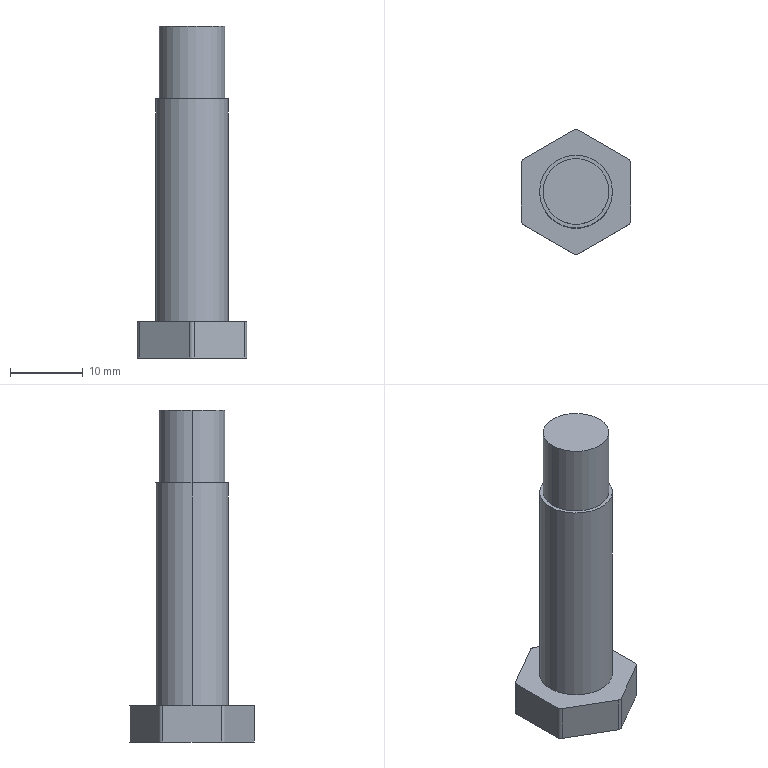Part | STEP file | Screw shaft QY-1-12 | 1 solid | 20 faces | box 15 x 17.135 x 45.5 mm | volume 4005 mm3 | cylinder 10 | plane 10 | commonest cylinder face diameters 1.2 x6 9 x2 10 x2
STEP:
#1=CARTESIAN_POINT('',(0.,0.,0.));
#2=DIRECTION('',(0.,0.,1.));
#3=DIRECTION('',(1.,0.,0.));
#4=AXIS2_PLACEMENT_3D('',#1,#2,#3);
#5=CARTESIAN_POINT('',(4.5,0.,30.5));
#6=VERTEX_POINT('',#5);
#7=CARTESIAN_POINT('',(-4.5,0.,30.5));
#8=VERTEX_POINT('',#7);
#9=CARTESIAN_POINT('',(0.,0.,30.5));
#10=DIRECTION('',(0.,0.,1.));
#11=DIRECTION('',(1.,0.,0.));
#12=AXIS2_PLACEMENT_3D('',#9,#10,#11);
#13=CIRCLE('',#12,4.5);
#14=CARTESIAN_POINT('',(0.,0.,30.5));
#15=DIRECTION('',(0.,0.,1.));
#16=DIRECTION('',(1.,0.,0.));
#17=AXIS2_PLACEMENT_3D('',#14,#15,#16);
#18=CYLINDRICAL_SURFACE('',#17,4.5);
#19=CARTESIAN_POINT('',(0.,0.));
#20=DIRECTION('',(1.,0.));
#21=VECTOR('',#20,1.);
#22=LINE('',#19,#21);
#23=(GEOMETRIC_REPRESENTATION_CONTEXT(2)PARAMETRIC_REPRESENTATION_CONTEXT()REPRESENTATION_CONTEXT('',''));
#24=DEFINITIONAL_REPRESENTATION('',(#22),#23);
#25=PCURVE('',#18,#24);
#26=CARTESIAN_POINT('',(0.,0.,30.5));
#27=DIRECTION('',(0.,0.,1.));
#28=DIRECTION('',(1.,0.,0.));
#29=AXIS2_PLACEMENT_3D('',#26,#27,#28);
#30=PLANE('',#29);
#31=CARTESIAN_POINT('',(0.,0.));
#32=DIRECTION('',(1.,0.));
#33=AXIS2_PLACEMENT_2D('',#31,#32);
#34=CIRCLE('',#33,4.5);
#35=(GEOMETRIC_REPRESENTATION_CONTEXT(2)PARAMETRIC_REPRESENTATION_CONTEXT()REPRESENTATION_CONTEXT('',''));
#36=DEFINITIONAL_REPRESENTATION('',(#34),#35);
#37=PCURVE('',#30,#36);
#38=SURFACE_CURVE('',#13,(#25,#37),.PCURVE_S1.);
#39=EDGE_CURVE('',#6,#8,#38,.T.);
#40=ORIENTED_EDGE('',*,*,#39,.T.);
#41=CARTESIAN_POINT('',(-4.5,0.,40.5));
#42=VERTEX_POINT('',#41);
#43=CARTESIAN_POINT('',(-4.5,0.,30.5));
#44=DIRECTION('',(0.,0.,1.));
#45=VECTOR('',#44,1.);
#46=LINE('',#43,#45);
#47=CARTESIAN_POINT('',(3.142,0.));
#48=DIRECTION('',(0.,1.));
#49=VECTOR('',#48,1.);
#50=LINE('',#47,#49);
#51=(GEOMETRIC_REPRESENTATION_CONTEXT(2)PARAMETRIC_REPRESENTATION_CONTEXT()REPRESENTATION_CONTEXT('',''));
#52=DEFINITIONAL_REPRESENTATION('',(#50),#51);
#53=PCURVE('',#18,#52);
#54=CARTESIAN_POINT('',(0.,0.,30.5));
#55=DIRECTION('',(0.,0.,1.));
#56=DIRECTION('',(1.,0.,0.));
#57=AXIS2_PLACEMENT_3D('',#54,#55,#56);
#58=CYLINDRICAL_SURFACE('',#57,4.5);
#59=CARTESIAN_POINT('',(3.142,0.));
#60=DIRECTION('',(0.,1.));
#61=VECTOR('',#60,1.);
#62=LINE('',#59,#61);
#63=(GEOMETRIC_REPRESENTATION_CONTEXT(2)PARAMETRIC_REPRESENTATION_CONTEXT()REPRESENTATION_CONTEXT('',''));
#64=DEFINITIONAL_REPRESENTATION('',(#62),#63);
#65=PCURVE('',#58,#64);
#66=SURFACE_CURVE('',#46,(#53,#65),.PCURVE_S1.);
#67=EDGE_CURVE('',#8,#42,#66,.T.);
#68=ORIENTED_EDGE('',*,*,#67,.T.);
#69=CARTESIAN_POINT('',(4.5,0.,40.5));
#70=VERTEX_POINT('',#69);
#71=CARTESIAN_POINT('',(0.,0.,40.5));
#72=DIRECTION('',(0.,0.,1.));
#73=DIRECTION('',(1.,0.,0.));
#74=AXIS2_PLACEMENT_3D('',#71,#72,#73);
#75=CIRCLE('',#74,4.5);
#76=CARTESIAN_POINT('',(0.,10.));
#77=DIRECTION('',(1.,0.));
#78=VECTOR('',#77,1.);
#79=LINE('',#76,#78);
#80=(GEOMETRIC_REPRESENTATION_CONTEXT(2)PARAMETRIC_REPRESENTATION_CONTEXT()REPRESENTATION_CONTEXT('',''));
#81=DEFINITIONAL_REPRESENTATION('',(#79),#80);
#82=PCURVE('',#18,#81);
#83=CARTESIAN_POINT('',(0.,0.,40.5));
#84=DIRECTION('',(0.,0.,1.));
#85=DIRECTION('',(1.,0.,0.));
#86=AXIS2_PLACEMENT_3D('',#83,#84,#85);
#87=PLANE('',#86);
#88=CARTESIAN_POINT('',(0.,0.));
#89=DIRECTION('',(1.,0.));
#90=AXIS2_PLACEMENT_2D('',#88,#89);
#91=CIRCLE('',#90,4.5);
#92=(GEOMETRIC_REPRESENTATION_CONTEXT(2)PARAMETRIC_REPRESENTATION_CONTEXT()REPRESENTATION_CONTEXT('',''));
#93=DEFINITIONAL_REPRESENTATION('',(#91),#92);
#94=PCURVE('',#87,#93);
#95=SURFACE_CURVE('',#75,(#82,#94),.PCURVE_S1.);
#96=EDGE_CURVE('',#70,#42,#95,.T.);
#97=ORIENTED_EDGE('',*,*,#96,.F.);
#98=CARTESIAN_POINT('',(4.5,0.,30.5));
#99=DIRECTION('',(0.,0.,1.));
#100=VECTOR('',#99,1.);
#101=LINE('',#98,#100);
#102=CARTESIAN_POINT('',(0.,0.));
#103=DIRECTION('',(0.,1.));
#104=VECTOR('',#103,1.);
#105=LINE('',#102,#104);
#106=(GEOMETRIC_REPRESENTATION_CONTEXT(2)PARAMETRIC_REPRESENTATION_CONTEXT()REPRESENTATION_CONTEXT('',''));
#107=DEFINITIONAL_REPRESENTATION('',(#105),#106);
#108=PCURVE('',#18,#107);
#109=CARTESIAN_POINT('',(6.283,0.));
#110=DIRECTION('',(0.,1.));
#111=VECTOR('',#110,1.);
#112=LINE('',#109,#111);
#113=(GEOMETRIC_REPRESENTATION_CONTEXT(2)PARAMETRIC_REPRESENTATION_CONTEXT()REPRESENTATION_CONTEXT('',''));
#114=DEFINITIONAL_REPRESENTATION('',(#112),#113);
#115=PCURVE('',#58,#114);
#116=SURFACE_CURVE('',#101,(#108,#115),.PCURVE_S1.);
#117=EDGE_CURVE('',#6,#70,#116,.T.);
#118=ORIENTED_EDGE('',*,*,#117,.F.);
#119=EDGE_LOOP('',(#40,#68,#97,#118));
#120=FACE_BOUND('',#119,.T.);
#121=ADVANCED_FACE('',(#120),#18,.T.);
#122=CARTESIAN_POINT('',(5.,0.,30.5));
#123=VERTEX_POINT('',#122);
#124=CARTESIAN_POINT('',(-5.,0.,30.5));
#125=VERTEX_POINT('',#124);
#126=CARTESIAN_POINT('',(0.,0.,30.5));
#127=DIRECTION('',(0.,0.,1.));
#128=DIRECTION('',(1.,0.,0.));
#129=AXIS2_PLACEMENT_3D('',#126,#127,#128);
#130=CIRCLE('',#129,5.);
#131=CARTESIAN_POINT('',(0.,0.,36.5));
#132=DIRECTION('',(0.,0.,-1.));
#133=DIRECTION('',(-1.,0.,0.));
#134=AXIS2_PLACEMENT_3D('',#131,#132,#133);
#135=CYLINDRICAL_SURFACE('',#134,5.);
#136=CARTESIAN_POINT('',(3.142,6.));
#137=DIRECTION('',(-1.,0.));
#138=VECTOR('',#137,1.);
#139=LINE('',#136,#138);
#140=(GEOMETRIC_REPRESENTATION_CONTEXT(2)PARAMETRIC_REPRESENTATION_CONTEXT()REPRESENTATION_CONTEXT('',''));
#141=DEFINITIONAL_REPRESENTATION('',(#139),#140);
#142=PCURVE('',#135,#141);
#143=CARTESIAN_POINT('',(0.,0.));
#144=DIRECTION('',(1.,0.));
#145=AXIS2_PLACEMENT_2D('',#143,#144);
#146=CIRCLE('',#145,5.);
#147=(GEOMETRIC_REPRESENTATION_CONTEXT(2)PARAMETRIC_REPRESENTATION_CONTEXT()REPRESENTATION_CONTEXT('',''));
#148=DEFINITIONAL_REPRESENTATION('',(#146),#147);
#149=PCURVE('',#30,#148);
#150=SURFACE_CURVE('',#130,(#142,#149),.PCURVE_S1.);
#151=EDGE_CURVE('',#123,#125,#150,.T.);
#152=ORIENTED_EDGE('',*,*,#151,.F.);
#153=CARTESIAN_POINT('',(5.,0.,0.));
#154=VERTEX_POINT('',#153);
#155=CARTESIAN_POINT('',(5.,0.,36.5));
#156=DIRECTION('',(0.,0.,-1.));
#157=VECTOR('',#156,1.);
#158=LINE('',#155,#157);
#159=CARTESIAN_POINT('',(3.142,0.));
#160=DIRECTION('',(0.,1.));
#161=VECTOR('',#160,1.);
#162=LINE('',#159,#161);
#163=(GEOMETRIC_REPRESENTATION_CONTEXT(2)PARAMETRIC_REPRESENTATION_CONTEXT()REPRESENTATION_CONTEXT('',''));
#164=DEFINITIONAL_REPRESENTATION('',(#162),#163);
#165=PCURVE('',#135,#164);
#166=CARTESIAN_POINT('',(0.,0.,36.5));
#167=DIRECTION('',(0.,0.,-1.));
#168=DIRECTION('',(-1.,0.,0.));
#169=AXIS2_PLACEMENT_3D('',#166,#167,#168);
#170=CYLINDRICAL_SURFACE('',#169,5.);
#171=CARTESIAN_POINT('',(3.142,0.));
#172=DIRECTION('',(0.,1.));
#173=VECTOR('',#172,1.);
#174=LINE('',#171,#173);
#175=(GEOMETRIC_REPRESENTATION_CONTEXT(2)PARAMETRIC_REPRESENTATION_CONTEXT()REPRESENTATION_CONTEXT('',''));
#176=DEFINITIONAL_REPRESENTATION('',(#174),#175);
#177=PCURVE('',#170,#176);
#178=SURFACE_CURVE('',#158,(#165,#177),.PCURVE_S1.);
#179=EDGE_CURVE('',#123,#154,#178,.T.);
#180=ORIENTED_EDGE('',*,*,#179,.T.);
#181=CARTESIAN_POINT('',(-5.,0.,0.));
#182=VERTEX_POINT('',#181);
#183=CARTESIAN_POINT('',(0.,0.,0.));
#184=DIRECTION('',(0.,0.,1.));
#185=DIRECTION('',(1.,0.,0.));
#186=AXIS2_PLACEMENT_3D('',#183,#184,#185);
#187=CIRCLE('',#186,5.);
#188=CARTESIAN_POINT('',(3.142,36.5));
#189=DIRECTION('',(-1.,0.));
#190=VECTOR('',#189,1.);
#191=LINE('',#188,#190);
#192=(GEOMETRIC_REPRESENTATION_CONTEXT(2)PARAMETRIC_REPRESENTATION_CONTEXT()REPRESENTATION_CONTEXT('',''));
#193=DEFINITIONAL_REPRESENTATION('',(#191),#192);
#194=PCURVE('',#135,#193);
#195=CARTESIAN_POINT('',(-6.9,3.984,0.));
#196=DIRECTION('',(0.,0.,-1.));
#197=DIRECTION('',(-1.,0.,0.));
#198=AXIS2_PLACEMENT_3D('',#195,#196,#197);
#199=PLANE('',#198);
#200=CARTESIAN_POINT('',(-11.9,-3.984));
#201=CARTESIAN_POINT('',(-11.9,4.677));
#202=CARTESIAN_POINT('',(-4.4,0.3464));
#203=CARTESIAN_POINT('',(3.1,-3.984));
#204=CARTESIAN_POINT('',(-4.4,-8.314));
#205=CARTESIAN_POINT('',(-11.9,-12.644));
#206=CARTESIAN_POINT('',(-11.9,-3.984));
#207=(BOUNDED_CURVE()B_SPLINE_CURVE(2,(#200,#201,#202,#203,#204,#205,#206),.UNSPECIFIED.,.T.,.F.)B_SPLINE_CURVE_WITH_KNOTS((1,2,2,2,2,1),(-2.094,0.,2.094,4.189,6.283,8.378),.UNSPECIFIED.)CURVE()GEOMETRIC_REPRESENTATION_ITEM()RATIONAL_B_SPLINE_CURVE((1.,0.5,1.,0.5,1.,0.5,1.))REPRESENTATION_ITEM(''));
#208=(GEOMETRIC_REPRESENTATION_CONTEXT(2)PARAMETRIC_REPRESENTATION_CONTEXT()REPRESENTATION_CONTEXT('',''));
#209=DEFINITIONAL_REPRESENTATION('',(#207),#208);
#210=PCURVE('',#199,#209);
#211=SURFACE_CURVE('',#187,(#194,#210),.PCURVE_S1.);
#212=EDGE_CURVE('',#154,#182,#211,.T.);
#213=ORIENTED_EDGE('',*,*,#212,.T.);
#214=CARTESIAN_POINT('',(-5.,0.,36.5));
#215=DIRECTION('',(0.,0.,-1.));
#216=VECTOR('',#215,1.);
#217=LINE('',#214,#216);
#218=CARTESIAN_POINT('',(0.,0.));
#219=DIRECTION('',(0.,1.));
#220=VECTOR('',#219,1.);
#221=LINE('',#218,#220);
#222=(GEOMETRIC_REPRESENTATION_CONTEXT(2)PARAMETRIC_REPRESENTATION_CONTEXT()REPRESENTATION_CONTEXT('',''));
#223=DEFINITIONAL_REPRESENTATION('',(#221),#222);
#224=PCURVE('',#135,#223);
#225=CARTESIAN_POINT('',(6.283,0.));
#226=DIRECTION('',(0.,1.));
#227=VECTOR('',#226,1.);
#228=LINE('',#225,#227);
#229=(GEOMETRIC_REPRESENTATION_CONTEXT(2)PARAMETRIC_REPRESENTATION_CONTEXT()REPRESENTATION_CONTEXT('',''));
#230=DEFINITIONAL_REPRESENTATION('',(#228),#229);
#231=PCURVE('',#170,#230);
#232=SURFACE_CURVE('',#217,(#224,#231),.PCURVE_S1.);
#233=EDGE_CURVE('',#125,#182,#232,.T.);
#234=ORIENTED_EDGE('',*,*,#233,.F.);
#235=EDGE_LOOP('',(#152,#180,#213,#234));
#236=FACE_BOUND('',#235,.T.);
#237=ADVANCED_FACE('',(#236),#135,.T.);
#238=ORIENTED_EDGE('',*,*,#179,.F.);
#239=CARTESIAN_POINT('',(0.,0.,30.5));
#240=DIRECTION('',(0.,0.,1.));
#241=DIRECTION('',(1.,0.,0.));
#242=AXIS2_PLACEMENT_3D('',#239,#240,#241);
#243=CIRCLE('',#242,5.);
#244=CARTESIAN_POINT('',(9.425,6.));
#245=DIRECTION('',(-1.,0.));
#246=VECTOR('',#245,1.);
#247=LINE('',#244,#246);
#248=(GEOMETRIC_REPRESENTATION_CONTEXT(2)PARAMETRIC_REPRESENTATION_CONTEXT()REPRESENTATION_CONTEXT('',''));
#249=DEFINITIONAL_REPRESENTATION('',(#247),#248);
#250=PCURVE('',#170,#249);
#251=CARTESIAN_POINT('',(0.,0.));
#252=DIRECTION('',(1.,0.));
#253=AXIS2_PLACEMENT_2D('',#251,#252);
#254=CIRCLE('',#253,5.);
#255=(GEOMETRIC_REPRESENTATION_CONTEXT(2)PARAMETRIC_REPRESENTATION_CONTEXT()REPRESENTATION_CONTEXT('',''));
#256=DEFINITIONAL_REPRESENTATION('',(#254),#255);
#257=PCURVE('',#30,#256);
#258=SURFACE_CURVE('',#243,(#250,#257),.PCURVE_S1.);
#259=EDGE_CURVE('',#125,#123,#258,.T.);
#260=ORIENTED_EDGE('',*,*,#259,.F.);
#261=ORIENTED_EDGE('',*,*,#233,.T.);
#262=CARTESIAN_POINT('',(0.,0.,0.));
#263=DIRECTION('',(0.,0.,1.));
#264=DIRECTION('',(1.,0.,0.));
#265=AXIS2_PLACEMENT_3D('',#262,#263,#264);
#266=CIRCLE('',#265,5.);
#267=CARTESIAN_POINT('',(9.425,36.5));
#268=DIRECTION('',(-1.,0.));
#269=VECTOR('',#268,1.);
#270=LINE('',#267,#269);
#271=(GEOMETRIC_REPRESENTATION_CONTEXT(2)PARAMETRIC_REPRESENTATION_CONTEXT()REPRESENTATION_CONTEXT('',''));
#272=DEFINITIONAL_REPRESENTATION('',(#270),#271);
#273=PCURVE('',#170,#272);
#274=CARTESIAN_POINT('',(-11.9,-3.984));
#275=CARTESIAN_POINT('',(-11.9,4.677));
#276=CARTESIAN_POINT('',(-4.4,0.3464));
#277=CARTESIAN_POINT('',(3.1,-3.984));
#278=CARTESIAN_POINT('',(-4.4,-8.314));
#279=CARTESIAN_POINT('',(-11.9,-12.644));
#280=CARTESIAN_POINT('',(-11.9,-3.984));
#281=(BOUNDED_CURVE()B_SPLINE_CURVE(2,(#274,#275,#276,#277,#278,#279,#280),.UNSPECIFIED.,.T.,.F.)B_SPLINE_CURVE_WITH_KNOTS((1,2,2,2,2,1),(-2.094,0.,2.094,4.189,6.283,8.378),.UNSPECIFIED.)CURVE()GEOMETRIC_REPRESENTATION_ITEM()RATIONAL_B_SPLINE_CURVE((1.,0.5,1.,0.5,1.,0.5,1.))REPRESENTATION_ITEM(''));
#282=(GEOMETRIC_REPRESENTATION_CONTEXT(2)PARAMETRIC_REPRESENTATION_CONTEXT()REPRESENTATION_CONTEXT('',''));
#283=DEFINITIONAL_REPRESENTATION('',(#281),#282);
#284=PCURVE('',#199,#283);
#285=SURFACE_CURVE('',#266,(#273,#284),.PCURVE_S1.);
#286=EDGE_CURVE('',#182,#154,#285,.T.);
#287=ORIENTED_EDGE('',*,*,#286,.T.);
#288=EDGE_LOOP('',(#238,#260,#261,#287));
#289=FACE_BOUND('',#288,.T.);
#290=ADVANCED_FACE('',(#289),#170,.T.);
#291=CARTESIAN_POINT('',(-7.5,3.984,0.));
#292=VERTEX_POINT('',#291);
#293=CARTESIAN_POINT('',(-7.2,4.503,0.));
#294=VERTEX_POINT('',#293);
#295=CARTESIAN_POINT('',(-6.9,3.984,0.));
#296=DIRECTION('',(0.,0.,-1.));
#297=DIRECTION('',(-1.,0.,0.));
#298=AXIS2_PLACEMENT_3D('',#295,#296,#297);
#299=CIRCLE('',#298,0.6);
#300=CARTESIAN_POINT('',(-6.9,3.984,-5.));
#301=DIRECTION('',(0.,0.,1.));
#302=DIRECTION('',(1.,0.,0.));
#303=AXIS2_PLACEMENT_3D('',#300,#301,#302);
#304=CYLINDRICAL_SURFACE('',#303,0.6);
#305=CARTESIAN_POINT('',(3.142,5.));
#306=DIRECTION('',(-1.,0.));
#307=VECTOR('',#306,1.);
#308=LINE('',#305,#307);
#309=(GEOMETRIC_REPRESENTATION_CONTEXT(2)PARAMETRIC_REPRESENTATION_CONTEXT()REPRESENTATION_CONTEXT('',''));
#310=DEFINITIONAL_REPRESENTATION('',(#308),#309);
#311=PCURVE('',#304,#310);
#312=CARTESIAN_POINT('',(0.,0.));
#313=DIRECTION('',(1.,0.));
#314=AXIS2_PLACEMENT_2D('',#312,#313);
#315=CIRCLE('',#314,0.6);
#316=(GEOMETRIC_REPRESENTATION_CONTEXT(2)PARAMETRIC_REPRESENTATION_CONTEXT()REPRESENTATION_CONTEXT('',''));
#317=DEFINITIONAL_REPRESENTATION('',(#315),#316);
#318=PCURVE('',#199,#317);
#319=SURFACE_CURVE('',#299,(#311,#318),.PCURVE_S1.);
#320=EDGE_CURVE('',#292,#294,#319,.T.);
#321=ORIENTED_EDGE('',*,*,#320,.T.);
#322=CARTESIAN_POINT('',(-7.2,4.503,-5.));
#323=VERTEX_POINT('',#322);
#324=CARTESIAN_POINT('',(-7.2,4.503,-5.));
#325=DIRECTION('',(0.,0.,1.));
#326=VECTOR('',#325,1.);
#327=LINE('',#324,#326);
#328=CARTESIAN_POINT('',(2.094,0.));
#329=DIRECTION('',(0.,1.));
#330=VECTOR('',#329,1.);
#331=LINE('',#328,#330);
#332=(GEOMETRIC_REPRESENTATION_CONTEXT(2)PARAMETRIC_REPRESENTATION_CONTEXT()REPRESENTATION_CONTEXT('',''));
#333=DEFINITIONAL_REPRESENTATION('',(#331),#332);
#334=PCURVE('',#304,#333);
#335=CARTESIAN_POINT('',(-7.2,4.503,-5.));
#336=DIRECTION('',(0.5,-0.866,0.));
#337=DIRECTION('',(0.866,0.5,0.));
#338=AXIS2_PLACEMENT_3D('',#335,#336,#337);
#339=PLANE('',#338);
#340=CARTESIAN_POINT('',(0.,0.));
#341=DIRECTION('',(0.,1.));
#342=VECTOR('',#341,1.);
#343=LINE('',#340,#342);
#344=(GEOMETRIC_REPRESENTATION_CONTEXT(2)PARAMETRIC_REPRESENTATION_CONTEXT()REPRESENTATION_CONTEXT('',''));
#345=DEFINITIONAL_REPRESENTATION('',(#343),#344);
#346=PCURVE('',#339,#345);
#347=SURFACE_CURVE('',#327,(#334,#346),.PCURVE_S1.);
#348=EDGE_CURVE('',#323,#294,#347,.T.);
#349=ORIENTED_EDGE('',*,*,#348,.F.);
#350=CARTESIAN_POINT('',(-7.5,3.984,-5.));
#351=VERTEX_POINT('',#350);
#352=CARTESIAN_POINT('',(-6.9,3.984,-5.));
#353=DIRECTION('',(0.,0.,-1.));
#354=DIRECTION('',(-1.,0.,0.));
#355=AXIS2_PLACEMENT_3D('',#352,#353,#354);
#356=CIRCLE('',#355,0.6);
#357=CARTESIAN_POINT('',(3.142,0.));
#358=DIRECTION('',(-1.,0.));
#359=VECTOR('',#358,1.);
#360=LINE('',#357,#359);
#361=(GEOMETRIC_REPRESENTATION_CONTEXT(2)PARAMETRIC_REPRESENTATION_CONTEXT()REPRESENTATION_CONTEXT('',''));
#362=DEFINITIONAL_REPRESENTATION('',(#360),#361);
#363=PCURVE('',#304,#362);
#364=CARTESIAN_POINT('',(-6.9,3.984,-5.));
#365=DIRECTION('',(0.,0.,-1.));
#366=DIRECTION('',(-1.,0.,0.));
#367=AXIS2_PLACEMENT_3D('',#364,#365,#366);
#368=PLANE('',#367);
#369=CARTESIAN_POINT('',(0.,0.));
#370=DIRECTION('',(1.,0.));
#371=AXIS2_PLACEMENT_2D('',#369,#370);
#372=CIRCLE('',#371,0.6);
#373=(GEOMETRIC_REPRESENTATION_CONTEXT(2)PARAMETRIC_REPRESENTATION_CONTEXT()REPRESENTATION_CONTEXT('',''));
#374=DEFINITIONAL_REPRESENTATION('',(#372),#373);
#375=PCURVE('',#368,#374);
#376=SURFACE_CURVE('',#356,(#363,#375),.PCURVE_S1.);
#377=EDGE_CURVE('',#351,#323,#376,.T.);
#378=ORIENTED_EDGE('',*,*,#377,.F.);
#379=CARTESIAN_POINT('',(-7.5,3.984,-5.));
#380=DIRECTION('',(0.,0.,1.));
#381=VECTOR('',#380,1.);
#382=LINE('',#379,#381);
#383=CARTESIAN_POINT('',(3.142,0.));
#384=DIRECTION('',(0.,1.));
#385=VECTOR('',#384,1.);
#386=LINE('',#383,#385);
#387=(GEOMETRIC_REPRESENTATION_CONTEXT(2)PARAMETRIC_REPRESENTATION_CONTEXT()REPRESENTATION_CONTEXT('',''));
#388=DEFINITIONAL_REPRESENTATION('',(#386),#387);
#389=PCURVE('',#304,#388);
#390=CARTESIAN_POINT('',(-7.5,-3.984,-5.));
#391=DIRECTION('',(1.,0.,0.));
#392=DIRECTION('',(0.,1.,0.));
#393=AXIS2_PLACEMENT_3D('',#390,#391,#392);
#394=PLANE('',#393);
#395=CARTESIAN_POINT('',(7.967,0.));
#396=DIRECTION('',(0.,1.));
#397=VECTOR('',#396,1.);
#398=LINE('',#395,#397);
#399=(GEOMETRIC_REPRESENTATION_CONTEXT(2)PARAMETRIC_REPRESENTATION_CONTEXT()REPRESENTATION_CONTEXT('',''));
#400=DEFINITIONAL_REPRESENTATION('',(#398),#399);
#401=PCURVE('',#394,#400);
#402=SURFACE_CURVE('',#382,(#389,#401),.PCURVE_S1.);
#403=EDGE_CURVE('',#351,#292,#402,.T.);
#404=ORIENTED_EDGE('',*,*,#403,.T.);
#405=EDGE_LOOP('',(#321,#349,#378,#404));
#406=FACE_BOUND('',#405,.T.);
#407=ADVANCED_FACE('',(#406),#304,.T.);
#408=CARTESIAN_POINT('',(-0.3,8.487,0.));
#409=VERTEX_POINT('',#408);
#410=CARTESIAN_POINT('',(-7.2,4.503,0.));
#411=DIRECTION('',(0.866,0.5,0.));
#412=VECTOR('',#411,1.);
#413=LINE('',#410,#412);
#414=CARTESIAN_POINT('',(0.,5.));
#415=DIRECTION('',(1.,0.));
#416=VECTOR('',#415,1.);
#417=LINE('',#414,#416);
#418=(GEOMETRIC_REPRESENTATION_CONTEXT(2)PARAMETRIC_REPRESENTATION_CONTEXT()REPRESENTATION_CONTEXT('',''));
#419=DEFINITIONAL_REPRESENTATION('',(#417),#418);
#420=PCURVE('',#339,#419);
#421=CARTESIAN_POINT('',(0.3,0.5196));
#422=DIRECTION('',(-0.866,0.5));
#423=VECTOR('',#422,1.);
#424=LINE('',#421,#423);
#425=(GEOMETRIC_REPRESENTATION_CONTEXT(2)PARAMETRIC_REPRESENTATION_CONTEXT()REPRESENTATION_CONTEXT('',''));
#426=DEFINITIONAL_REPRESENTATION('',(#424),#425);
#427=PCURVE('',#199,#426);
#428=SURFACE_CURVE('',#413,(#420,#427),.PCURVE_S1.);
#429=EDGE_CURVE('',#294,#409,#428,.T.);
#430=ORIENTED_EDGE('',*,*,#429,.T.);
#431=CARTESIAN_POINT('',(-0.3,8.487,-5.));
#432=VERTEX_POINT('',#431);
#433=CARTESIAN_POINT('',(-0.3,8.487,-5.));
#434=DIRECTION('',(0.,0.,1.));
#435=VECTOR('',#434,1.);
#436=LINE('',#433,#435);
#437=CARTESIAN_POINT('',(7.967,0.));
#438=DIRECTION('',(0.,1.));
#439=VECTOR('',#438,1.);
#440=LINE('',#437,#439);
#441=(GEOMETRIC_REPRESENTATION_CONTEXT(2)PARAMETRIC_REPRESENTATION_CONTEXT()REPRESENTATION_CONTEXT('',''));
#442=DEFINITIONAL_REPRESENTATION('',(#440),#441);
#443=PCURVE('',#339,#442);
#444=CARTESIAN_POINT('',(0.,7.967,-5.));
#445=DIRECTION('',(0.,0.,1.));
#446=DIRECTION('',(1.,0.,0.));
#447=AXIS2_PLACEMENT_3D('',#444,#445,#446);
#448=CYLINDRICAL_SURFACE('',#447,0.6);
#449=CARTESIAN_POINT('',(2.094,0.));
#450=DIRECTION('',(0.,1.));
#451=VECTOR('',#450,1.);
#452=LINE('',#449,#451);
#453=(GEOMETRIC_REPRESENTATION_CONTEXT(2)PARAMETRIC_REPRESENTATION_CONTEXT()REPRESENTATION_CONTEXT('',''));
#454=DEFINITIONAL_REPRESENTATION('',(#452),#453);
#455=PCURVE('',#448,#454);
#456=SURFACE_CURVE('',#436,(#443,#455),.PCURVE_S1.);
#457=EDGE_CURVE('',#432,#409,#456,.T.);
#458=ORIENTED_EDGE('',*,*,#457,.F.);
#459=CARTESIAN_POINT('',(-7.2,4.503,-5.));
#460=DIRECTION('',(0.866,0.5,0.));
#461=VECTOR('',#460,1.);
#462=LINE('',#459,#461);
#463=CARTESIAN_POINT('',(0.,0.));
#464=DIRECTION('',(1.,0.));
#465=VECTOR('',#464,1.);
#466=LINE('',#463,#465);
#467=(GEOMETRIC_REPRESENTATION_CONTEXT(2)PARAMETRIC_REPRESENTATION_CONTEXT()REPRESENTATION_CONTEXT('',''));
#468=DEFINITIONAL_REPRESENTATION('',(#466),#467);
#469=PCURVE('',#339,#468);
#470=CARTESIAN_POINT('',(0.3,0.5196));
#471=DIRECTION('',(-0.866,0.5));
#472=VECTOR('',#471,1.);
#473=LINE('',#470,#472);
#474=(GEOMETRIC_REPRESENTATION_CONTEXT(2)PARAMETRIC_REPRESENTATION_CONTEXT()REPRESENTATION_CONTEXT('',''));
#475=DEFINITIONAL_REPRESENTATION('',(#473),#474);
#476=PCURVE('',#368,#475);
#477=SURFACE_CURVE('',#462,(#469,#476),.PCURVE_S1.);
#478=EDGE_CURVE('',#323,#432,#477,.T.);
#479=ORIENTED_EDGE('',*,*,#478,.F.);
#480=ORIENTED_EDGE('',*,*,#348,.T.);
#481=EDGE_LOOP('',(#430,#458,#479,#480));
#482=FACE_BOUND('',#481,.T.);
#483=ADVANCED_FACE('',(#482),#339,.F.);
#484=CARTESIAN_POINT('',(0.3,8.487,0.));
#485=VERTEX_POINT('',#484);
#486=CARTESIAN_POINT('',(0.,7.967,0.));
#487=DIRECTION('',(0.,0.,-1.));
#488=DIRECTION('',(1.,0.,0.));
#489=AXIS2_PLACEMENT_3D('',#486,#487,#488);
#490=CIRCLE('',#489,0.6);
#491=CARTESIAN_POINT('',(6.283,5.));
#492=DIRECTION('',(-1.,0.));
#493=VECTOR('',#492,1.);
#494=LINE('',#491,#493);
#495=(GEOMETRIC_REPRESENTATION_CONTEXT(2)PARAMETRIC_REPRESENTATION_CONTEXT()REPRESENTATION_CONTEXT('',''));
#496=DEFINITIONAL_REPRESENTATION('',(#494),#495);
#497=PCURVE('',#448,#496);
#498=CARTESIAN_POINT('',(-6.9,3.984));
#499=DIRECTION('',(-1.,0.));
#500=AXIS2_PLACEMENT_2D('',#498,#499);
#501=CIRCLE('',#500,0.6);
#502=(GEOMETRIC_REPRESENTATION_CONTEXT(2)PARAMETRIC_REPRESENTATION_CONTEXT()REPRESENTATION_CONTEXT('',''));
#503=DEFINITIONAL_REPRESENTATION('',(#501),#502);
#504=PCURVE('',#199,#503);
#505=SURFACE_CURVE('',#490,(#497,#504),.PCURVE_S1.);
#506=EDGE_CURVE('',#409,#485,#505,.T.);
#507=ORIENTED_EDGE('',*,*,#506,.T.);
#508=CARTESIAN_POINT('',(0.3,8.487,-5.));
#509=VERTEX_POINT('',#508);
#510=CARTESIAN_POINT('',(0.3,8.487,-5.));
#511=DIRECTION('',(0.,0.,1.));
#512=VECTOR('',#511,1.);
#513=LINE('',#510,#512);
#514=CARTESIAN_POINT('',(1.047,0.));
#515=DIRECTION('',(0.,1.));
#516=VECTOR('',#515,1.);
#517=LINE('',#514,#516);
#518=(GEOMETRIC_REPRESENTATION_CONTEXT(2)PARAMETRIC_REPRESENTATION_CONTEXT()REPRESENTATION_CONTEXT('',''));
#519=DEFINITIONAL_REPRESENTATION('',(#517),#518);
#520=PCURVE('',#448,#519);
#521=CARTESIAN_POINT('',(0.3,8.487,-5.));
#522=DIRECTION('',(-0.5,-0.866,0.));
#523=DIRECTION('',(0.866,-0.5,0.));
#524=AXIS2_PLACEMENT_3D('',#521,#522,#523);
#525=PLANE('',#524);
#526=CARTESIAN_POINT('',(0.,0.));
#527=DIRECTION('',(0.,1.));
#528=VECTOR('',#527,1.);
#529=LINE('',#526,#528);
#530=(GEOMETRIC_REPRESENTATION_CONTEXT(2)PARAMETRIC_REPRESENTATION_CONTEXT()REPRESENTATION_CONTEXT('',''));
#531=DEFINITIONAL_REPRESENTATION('',(#529),#530);
#532=PCURVE('',#525,#531);
#533=SURFACE_CURVE('',#513,(#520,#532),.PCURVE_S1.);
#534=EDGE_CURVE('',#509,#485,#533,.T.);
#535=ORIENTED_EDGE('',*,*,#534,.F.);
#536=CARTESIAN_POINT('',(0.,7.967,-5.));
#537=DIRECTION('',(0.,0.,-1.));
#538=DIRECTION('',(1.,0.,0.));
#539=AXIS2_PLACEMENT_3D('',#536,#537,#538);
#540=CIRCLE('',#539,0.6);
#541=CARTESIAN_POINT('',(6.283,0.));
#542=DIRECTION('',(-1.,0.));
#543=VECTOR('',#542,1.);
#544=LINE('',#541,#543);
#545=(GEOMETRIC_REPRESENTATION_CONTEXT(2)PARAMETRIC_REPRESENTATION_CONTEXT()REPRESENTATION_CONTEXT('',''));
#546=DEFINITIONAL_REPRESENTATION('',(#544),#545);
#547=PCURVE('',#448,#546);
#548=CARTESIAN_POINT('',(-6.9,3.984));
#549=DIRECTION('',(-1.,0.));
#550=AXIS2_PLACEMENT_2D('',#548,#549);
#551=CIRCLE('',#550,0.6);
#552=(GEOMETRIC_REPRESENTATION_CONTEXT(2)PARAMETRIC_REPRESENTATION_CONTEXT()REPRESENTATION_CONTEXT('',''));
#553=DEFINITIONAL_REPRESENTATION('',(#551),#552);
#554=PCURVE('',#368,#553);
#555=SURFACE_CURVE('',#540,(#547,#554),.PCURVE_S1.);
#556=EDGE_CURVE('',#432,#509,#555,.T.);
#557=ORIENTED_EDGE('',*,*,#556,.F.);
#558=ORIENTED_EDGE('',*,*,#457,.T.);
#559=EDGE_LOOP('',(#507,#535,#557,#558));
#560=FACE_BOUND('',#559,.T.);
#561=ADVANCED_FACE('',(#560),#448,.T.);
#562=CARTESIAN_POINT('',(7.2,4.503,0.));
#563=VERTEX_POINT('',#562);
#564=CARTESIAN_POINT('',(0.3,8.487,0.));
#565=DIRECTION('',(0.866,-0.5,0.));
#566=VECTOR('',#565,1.);
#567=LINE('',#564,#566);
#568=CARTESIAN_POINT('',(0.,5.));
#569=DIRECTION('',(1.,0.));
#570=VECTOR('',#569,1.);
#571=LINE('',#568,#570);
#572=(GEOMETRIC_REPRESENTATION_CONTEXT(2)PARAMETRIC_REPRESENTATION_CONTEXT()REPRESENTATION_CONTEXT('',''));
#573=DEFINITIONAL_REPRESENTATION('',(#571),#572);
#574=PCURVE('',#525,#573);
#575=CARTESIAN_POINT('',(-7.2,4.503));
#576=DIRECTION('',(-0.866,-0.5));
#577=VECTOR('',#576,1.);
#578=LINE('',#575,#577);
#579=(GEOMETRIC_REPRESENTATION_CONTEXT(2)PARAMETRIC_REPRESENTATION_CONTEXT()REPRESENTATION_CONTEXT('',''));
#580=DEFINITIONAL_REPRESENTATION('',(#578),#579);
#581=PCURVE('',#199,#580);
#582=SURFACE_CURVE('',#567,(#574,#581),.PCURVE_S1.);
#583=EDGE_CURVE('',#485,#563,#582,.T.);
#584=ORIENTED_EDGE('',*,*,#583,.T.);
#585=CARTESIAN_POINT('',(7.2,4.503,-5.));
#586=VERTEX_POINT('',#585);
#587=CARTESIAN_POINT('',(7.2,4.503,-5.));
#588=DIRECTION('',(0.,0.,1.));
#589=VECTOR('',#588,1.);
#590=LINE('',#587,#589);
#591=CARTESIAN_POINT('',(7.967,0.));
#592=DIRECTION('',(0.,1.));
#593=VECTOR('',#592,1.);
#594=LINE('',#591,#593);
#595=(GEOMETRIC_REPRESENTATION_CONTEXT(2)PARAMETRIC_REPRESENTATION_CONTEXT()REPRESENTATION_CONTEXT('',''));
#596=DEFINITIONAL_REPRESENTATION('',(#594),#595);
#597=PCURVE('',#525,#596);
#598=CARTESIAN_POINT('',(6.9,3.984,-5.));
#599=DIRECTION('',(0.,0.,1.));
#600=DIRECTION('',(1.,0.,0.));
#601=AXIS2_PLACEMENT_3D('',#598,#599,#600);
#602=CYLINDRICAL_SURFACE('',#601,0.6);
#603=CARTESIAN_POINT('',(1.047,0.));
#604=DIRECTION('',(0.,1.));
#605=VECTOR('',#604,1.);
#606=LINE('',#603,#605);
#607=(GEOMETRIC_REPRESENTATION_CONTEXT(2)PARAMETRIC_REPRESENTATION_CONTEXT()REPRESENTATION_CONTEXT('',''));
#608=DEFINITIONAL_REPRESENTATION('',(#606),#607);
#609=PCURVE('',#602,#608);
#610=SURFACE_CURVE('',#590,(#597,#609),.PCURVE_S1.);
#611=EDGE_CURVE('',#586,#563,#610,.T.);
#612=ORIENTED_EDGE('',*,*,#611,.F.);
#613=CARTESIAN_POINT('',(0.3,8.487,-5.));
#614=DIRECTION('',(0.866,-0.5,0.));
#615=VECTOR('',#614,1.);
#616=LINE('',#613,#615);
#617=CARTESIAN_POINT('',(0.,0.));
#618=DIRECTION('',(1.,0.));
#619=VECTOR('',#618,1.);
#620=LINE('',#617,#619);
#621=(GEOMETRIC_REPRESENTATION_CONTEXT(2)PARAMETRIC_REPRESENTATION_CONTEXT()REPRESENTATION_CONTEXT('',''));
#622=DEFINITIONAL_REPRESENTATION('',(#620),#621);
#623=PCURVE('',#525,#622);
#624=CARTESIAN_POINT('',(-7.2,4.503));
#625=DIRECTION('',(-0.866,-0.5));
#626=VECTOR('',#625,1.);
#627=LINE('',#624,#626);
#628=(GEOMETRIC_REPRESENTATION_CONTEXT(2)PARAMETRIC_REPRESENTATION_CONTEXT()REPRESENTATION_CONTEXT('',''));
#629=DEFINITIONAL_REPRESENTATION('',(#627),#628);
#630=PCURVE('',#368,#629);
#631=SURFACE_CURVE('',#616,(#623,#630),.PCURVE_S1.);
#632=EDGE_CURVE('',#509,#586,#631,.T.);
#633=ORIENTED_EDGE('',*,*,#632,.F.);
#634=ORIENTED_EDGE('',*,*,#534,.T.);
#635=EDGE_LOOP('',(#584,#612,#633,#634));
#636=FACE_BOUND('',#635,.T.);
#637=ADVANCED_FACE('',(#636),#525,.F.);
#638=CARTESIAN_POINT('',(7.5,3.984,0.));
#639=VERTEX_POINT('',#638);
#640=CARTESIAN_POINT('',(6.9,3.984,0.));
#641=DIRECTION('',(0.,0.,-1.));
#642=DIRECTION('',(-1.,0.,0.));
#643=AXIS2_PLACEMENT_3D('',#640,#641,#642);
#644=CIRCLE('',#643,0.6);
#645=CARTESIAN_POINT('',(3.142,5.));
#646=DIRECTION('',(-1.,0.));
#647=VECTOR('',#646,1.);
#648=LINE('',#645,#647);
#649=(GEOMETRIC_REPRESENTATION_CONTEXT(2)PARAMETRIC_REPRESENTATION_CONTEXT()REPRESENTATION_CONTEXT('',''));
#650=DEFINITIONAL_REPRESENTATION('',(#648),#649);
#651=PCURVE('',#602,#650);
#652=CARTESIAN_POINT('',(-13.8,0.));
#653=DIRECTION('',(1.,0.));
#654=AXIS2_PLACEMENT_2D('',#652,#653);
#655=CIRCLE('',#654,0.6);
#656=(GEOMETRIC_REPRESENTATION_CONTEXT(2)PARAMETRIC_REPRESENTATION_CONTEXT()REPRESENTATION_CONTEXT('',''));
#657=DEFINITIONAL_REPRESENTATION('',(#655),#656);
#658=PCURVE('',#199,#657);
#659=SURFACE_CURVE('',#644,(#651,#658),.PCURVE_S1.);
#660=EDGE_CURVE('',#563,#639,#659,.T.);
#661=ORIENTED_EDGE('',*,*,#660,.T.);
#662=CARTESIAN_POINT('',(7.5,3.984,-5.));
#663=VERTEX_POINT('',#662);
#664=CARTESIAN_POINT('',(7.5,3.984,-5.));
#665=DIRECTION('',(0.,0.,1.));
#666=VECTOR('',#665,1.);
#667=LINE('',#664,#666);
#668=CARTESIAN_POINT('',(0.,0.));
#669=DIRECTION('',(0.,1.));
#670=VECTOR('',#669,1.);
#671=LINE('',#668,#670);
#672=(GEOMETRIC_REPRESENTATION_CONTEXT(2)PARAMETRIC_REPRESENTATION_CONTEXT()REPRESENTATION_CONTEXT('',''));
#673=DEFINITIONAL_REPRESENTATION('',(#671),#672);
#674=PCURVE('',#602,#673);
#675=CARTESIAN_POINT('',(7.5,3.984,-5.));
#676=DIRECTION('',(-1.,0.,0.));
#677=DIRECTION('',(0.,-1.,0.));
#678=AXIS2_PLACEMENT_3D('',#675,#676,#677);
#679=PLANE('',#678);
#680=CARTESIAN_POINT('',(0.,0.));
#681=DIRECTION('',(0.,1.));
#682=VECTOR('',#681,1.);
#683=LINE('',#680,#682);
#684=(GEOMETRIC_REPRESENTATION_CONTEXT(2)PARAMETRIC_REPRESENTATION_CONTEXT()REPRESENTATION_CONTEXT('',''));
#685=DEFINITIONAL_REPRESENTATION('',(#683),#684);
#686=PCURVE('',#679,#685);
#687=SURFACE_CURVE('',#667,(#674,#686),.PCURVE_S1.);
#688=EDGE_CURVE('',#663,#639,#687,.T.);
#689=ORIENTED_EDGE('',*,*,#688,.F.);
#690=CARTESIAN_POINT('',(6.9,3.984,-5.));
#691=DIRECTION('',(0.,0.,-1.));
#692=DIRECTION('',(-1.,0.,0.));
#693=AXIS2_PLACEMENT_3D('',#690,#691,#692);
#694=CIRCLE('',#693,0.6);
#695=CARTESIAN_POINT('',(3.142,0.));
#696=DIRECTION('',(-1.,0.));
#697=VECTOR('',#696,1.);
#698=LINE('',#695,#697);
#699=(GEOMETRIC_REPRESENTATION_CONTEXT(2)PARAMETRIC_REPRESENTATION_CONTEXT()REPRESENTATION_CONTEXT('',''));
#700=DEFINITIONAL_REPRESENTATION('',(#698),#699);
#701=PCURVE('',#602,#700);
#702=CARTESIAN_POINT('',(-13.8,0.));
#703=DIRECTION('',(1.,0.));
#704=AXIS2_PLACEMENT_2D('',#702,#703);
#705=CIRCLE('',#704,0.6);
#706=(GEOMETRIC_REPRESENTATION_CONTEXT(2)PARAMETRIC_REPRESENTATION_CONTEXT()REPRESENTATION_CONTEXT('',''));
#707=DEFINITIONAL_REPRESENTATION('',(#705),#706);
#708=PCURVE('',#368,#707);
#709=SURFACE_CURVE('',#694,(#701,#708),.PCURVE_S1.);
#710=EDGE_CURVE('',#586,#663,#709,.T.);
#711=ORIENTED_EDGE('',*,*,#710,.F.);
#712=ORIENTED_EDGE('',*,*,#611,.T.);
#713=EDGE_LOOP('',(#661,#689,#711,#712));
#714=FACE_BOUND('',#713,.T.);
#715=ADVANCED_FACE('',(#714),#602,.T.);
#716=CARTESIAN_POINT('',(7.5,-3.984,0.));
#717=VERTEX_POINT('',#716);
#718=CARTESIAN_POINT('',(7.5,3.984,0.));
#719=DIRECTION('',(0.,-1.,0.));
#720=VECTOR('',#719,1.);
#721=LINE('',#718,#720);
#722=CARTESIAN_POINT('',(0.,5.));
#723=DIRECTION('',(1.,0.));
#724=VECTOR('',#723,1.);
#725=LINE('',#722,#724);
#726=(GEOMETRIC_REPRESENTATION_CONTEXT(2)PARAMETRIC_REPRESENTATION_CONTEXT()REPRESENTATION_CONTEXT('',''));
#727=DEFINITIONAL_REPRESENTATION('',(#725),#726);
#728=PCURVE('',#679,#727);
#729=CARTESIAN_POINT('',(-14.4,0.));
#730=DIRECTION('',(0.,-1.));
#731=VECTOR('',#730,1.);
#732=LINE('',#729,#731);
#733=(GEOMETRIC_REPRESENTATION_CONTEXT(2)PARAMETRIC_REPRESENTATION_CONTEXT()REPRESENTATION_CONTEXT('',''));
#734=DEFINITIONAL_REPRESENTATION('',(#732),#733);
#735=PCURVE('',#199,#734);
#736=SURFACE_CURVE('',#721,(#728,#735),.PCURVE_S1.);
#737=EDGE_CURVE('',#639,#717,#736,.T.);
#738=ORIENTED_EDGE('',*,*,#737,.T.);
#739=CARTESIAN_POINT('',(7.5,-3.984,-5.));
#740=VERTEX_POINT('',#739);
#741=CARTESIAN_POINT('',(7.5,-3.984,-5.));
#742=DIRECTION('',(0.,0.,1.));
#743=VECTOR('',#742,1.);
#744=LINE('',#741,#743);
#745=CARTESIAN_POINT('',(7.967,0.));
#746=DIRECTION('',(0.,1.));
#747=VECTOR('',#746,1.);
#748=LINE('',#745,#747);
#749=(GEOMETRIC_REPRESENTATION_CONTEXT(2)PARAMETRIC_REPRESENTATION_CONTEXT()REPRESENTATION_CONTEXT('',''));
#750=DEFINITIONAL_REPRESENTATION('',(#748),#749);
#751=PCURVE('',#679,#750);
#752=CARTESIAN_POINT('',(6.9,-3.984,-5.));
#753=DIRECTION('',(0.,0.,1.));
#754=DIRECTION('',(1.,0.,0.));
#755=AXIS2_PLACEMENT_3D('',#752,#753,#754);
#756=CYLINDRICAL_SURFACE('',#755,0.6);
#757=CARTESIAN_POINT('',(6.283,0.));
#758=DIRECTION('',(0.,1.));
#759=VECTOR('',#758,1.);
#760=LINE('',#757,#759);
#761=(GEOMETRIC_REPRESENTATION_CONTEXT(2)PARAMETRIC_REPRESENTATION_CONTEXT()REPRESENTATION_CONTEXT('',''));
#762=DEFINITIONAL_REPRESENTATION('',(#760),#761);
#763=PCURVE('',#756,#762);
#764=SURFACE_CURVE('',#744,(#751,#763),.PCURVE_S1.);
#765=EDGE_CURVE('',#740,#717,#764,.T.);
#766=ORIENTED_EDGE('',*,*,#765,.F.);
#767=CARTESIAN_POINT('',(7.5,3.984,-5.));
#768=DIRECTION('',(0.,-1.,0.));
#769=VECTOR('',#768,1.);
#770=LINE('',#767,#769);
#771=CARTESIAN_POINT('',(0.,0.));
#772=DIRECTION('',(1.,0.));
#773=VECTOR('',#772,1.);
#774=LINE('',#771,#773);
#775=(GEOMETRIC_REPRESENTATION_CONTEXT(2)PARAMETRIC_REPRESENTATION_CONTEXT()REPRESENTATION_CONTEXT('',''));
#776=DEFINITIONAL_REPRESENTATION('',(#774),#775);
#777=PCURVE('',#679,#776);
#778=CARTESIAN_POINT('',(-14.4,0.));
#779=DIRECTION('',(0.,-1.));
#780=VECTOR('',#779,1.);
#781=LINE('',#778,#780);
#782=(GEOMETRIC_REPRESENTATION_CONTEXT(2)PARAMETRIC_REPRESENTATION_CONTEXT()REPRESENTATION_CONTEXT('',''));
#783=DEFINITIONAL_REPRESENTATION('',(#781),#782);
#784=PCURVE('',#368,#783);
#785=SURFACE_CURVE('',#770,(#777,#784),.PCURVE_S1.);
#786=EDGE_CURVE('',#663,#740,#785,.T.);
#787=ORIENTED_EDGE('',*,*,#786,.F.);
#788=ORIENTED_EDGE('',*,*,#688,.T.);
#789=EDGE_LOOP('',(#738,#766,#787,#788));
#790=FACE_BOUND('',#789,.T.);
#791=ADVANCED_FACE('',(#790),#679,.F.);
#792=CARTESIAN_POINT('',(7.2,-4.503,0.));
#793=VERTEX_POINT('',#792);
#794=CARTESIAN_POINT('',(6.9,-3.984,0.));
#795=DIRECTION('',(0.,0.,-1.));
#796=DIRECTION('',(-1.,0.,0.));
#797=AXIS2_PLACEMENT_3D('',#794,#795,#796);
#798=CIRCLE('',#797,0.6);
#799=CARTESIAN_POINT('',(9.425,5.));
#800=DIRECTION('',(-1.,0.));
#801=VECTOR('',#800,1.);
#802=LINE('',#799,#801);
#803=(GEOMETRIC_REPRESENTATION_CONTEXT(2)PARAMETRIC_REPRESENTATION_CONTEXT()REPRESENTATION_CONTEXT('',''));
#804=DEFINITIONAL_REPRESENTATION('',(#802),#803);
#805=PCURVE('',#756,#804);
#806=CARTESIAN_POINT('',(-13.8,-7.967));
#807=DIRECTION('',(1.,0.));
#808=AXIS2_PLACEMENT_2D('',#806,#807);
#809=CIRCLE('',#808,0.6);
#810=(GEOMETRIC_REPRESENTATION_CONTEXT(2)PARAMETRIC_REPRESENTATION_CONTEXT()REPRESENTATION_CONTEXT('',''));
#811=DEFINITIONAL_REPRESENTATION('',(#809),#810);
#812=PCURVE('',#199,#811);
#813=SURFACE_CURVE('',#798,(#805,#812),.PCURVE_S1.);
#814=EDGE_CURVE('',#717,#793,#813,.T.);
#815=ORIENTED_EDGE('',*,*,#814,.T.);
#816=CARTESIAN_POINT('',(7.2,-4.503,-5.));
#817=VERTEX_POINT('',#816);
#818=CARTESIAN_POINT('',(7.2,-4.503,-5.));
#819=DIRECTION('',(0.,0.,1.));
#820=VECTOR('',#819,1.);
#821=LINE('',#818,#820);
#822=CARTESIAN_POINT('',(5.236,0.));
#823=DIRECTION('',(0.,1.));
#824=VECTOR('',#823,1.);
#825=LINE('',#822,#824);
#826=(GEOMETRIC_REPRESENTATION_CONTEXT(2)PARAMETRIC_REPRESENTATION_CONTEXT()REPRESENTATION_CONTEXT('',''));
#827=DEFINITIONAL_REPRESENTATION('',(#825),#826);
#828=PCURVE('',#756,#827);
#829=CARTESIAN_POINT('',(7.2,-4.503,-5.));
#830=DIRECTION('',(-0.5,0.866,0.));
#831=DIRECTION('',(-0.866,-0.5,0.));
#832=AXIS2_PLACEMENT_3D('',#829,#830,#831);
#833=PLANE('',#832);
#834=CARTESIAN_POINT('',(0.,0.));
#835=DIRECTION('',(0.,1.));
#836=VECTOR('',#835,1.);
#837=LINE('',#834,#836);
#838=(GEOMETRIC_REPRESENTATION_CONTEXT(2)PARAMETRIC_REPRESENTATION_CONTEXT()REPRESENTATION_CONTEXT('',''));
#839=DEFINITIONAL_REPRESENTATION('',(#837),#838);
#840=PCURVE('',#833,#839);
#841=SURFACE_CURVE('',#821,(#828,#840),.PCURVE_S1.);
#842=EDGE_CURVE('',#817,#793,#841,.T.);
#843=ORIENTED_EDGE('',*,*,#842,.F.);
#844=CARTESIAN_POINT('',(6.9,-3.984,-5.));
#845=DIRECTION('',(0.,0.,-1.));
#846=DIRECTION('',(-1.,0.,0.));
#847=AXIS2_PLACEMENT_3D('',#844,#845,#846);
#848=CIRCLE('',#847,0.6);
#849=CARTESIAN_POINT('',(9.425,0.));
#850=DIRECTION('',(-1.,0.));
#851=VECTOR('',#850,1.);
#852=LINE('',#849,#851);
#853=(GEOMETRIC_REPRESENTATION_CONTEXT(2)PARAMETRIC_REPRESENTATION_CONTEXT()REPRESENTATION_CONTEXT('',''));
#854=DEFINITIONAL_REPRESENTATION('',(#852),#853);
#855=PCURVE('',#756,#854);
#856=CARTESIAN_POINT('',(-13.8,-7.967));
#857=DIRECTION('',(1.,0.));
#858=AXIS2_PLACEMENT_2D('',#856,#857);
#859=CIRCLE('',#858,0.6);
#860=(GEOMETRIC_REPRESENTATION_CONTEXT(2)PARAMETRIC_REPRESENTATION_CONTEXT()REPRESENTATION_CONTEXT('',''));
#861=DEFINITIONAL_REPRESENTATION('',(#859),#860);
#862=PCURVE('',#368,#861);
#863=SURFACE_CURVE('',#848,(#855,#862),.PCURVE_S1.);
#864=EDGE_CURVE('',#740,#817,#863,.T.);
#865=ORIENTED_EDGE('',*,*,#864,.F.);
#866=ORIENTED_EDGE('',*,*,#765,.T.);
#867=EDGE_LOOP('',(#815,#843,#865,#866));
#868=FACE_BOUND('',#867,.T.);
#869=ADVANCED_FACE('',(#868),#756,.T.);
#870=CARTESIAN_POINT('',(0.3,-8.487,0.));
#871=VERTEX_POINT('',#870);
#872=CARTESIAN_POINT('',(7.2,-4.503,0.));
#873=DIRECTION('',(-0.866,-0.5,0.));
#874=VECTOR('',#873,1.);
#875=LINE('',#872,#874);
#876=CARTESIAN_POINT('',(0.,5.));
#877=DIRECTION('',(1.,0.));
#878=VECTOR('',#877,1.);
#879=LINE('',#876,#878);
#880=(GEOMETRIC_REPRESENTATION_CONTEXT(2)PARAMETRIC_REPRESENTATION_CONTEXT()REPRESENTATION_CONTEXT('',''));
#881=DEFINITIONAL_REPRESENTATION('',(#879),#880);
#882=PCURVE('',#833,#881);
#883=CARTESIAN_POINT('',(-14.1,-8.487));
#884=DIRECTION('',(0.866,-0.5));
#885=VECTOR('',#884,1.);
#886=LINE('',#883,#885);
#887=(GEOMETRIC_REPRESENTATION_CONTEXT(2)PARAMETRIC_REPRESENTATION_CONTEXT()REPRESENTATION_CONTEXT('',''));
#888=DEFINITIONAL_REPRESENTATION('',(#886),#887);
#889=PCURVE('',#199,#888);
#890=SURFACE_CURVE('',#875,(#882,#889),.PCURVE_S1.);
#891=EDGE_CURVE('',#793,#871,#890,.T.);
#892=ORIENTED_EDGE('',*,*,#891,.T.);
#893=CARTESIAN_POINT('',(0.3,-8.487,-5.));
#894=VERTEX_POINT('',#893);
#895=CARTESIAN_POINT('',(0.3,-8.487,-5.));
#896=DIRECTION('',(0.,0.,1.));
#897=VECTOR('',#896,1.);
#898=LINE('',#895,#897);
#899=CARTESIAN_POINT('',(7.967,0.));
#900=DIRECTION('',(0.,1.));
#901=VECTOR('',#900,1.);
#902=LINE('',#899,#901);
#903=(GEOMETRIC_REPRESENTATION_CONTEXT(2)PARAMETRIC_REPRESENTATION_CONTEXT()REPRESENTATION_CONTEXT('',''));
#904=DEFINITIONAL_REPRESENTATION('',(#902),#903);
#905=PCURVE('',#833,#904);
#906=CARTESIAN_POINT('',(0.,-7.967,-5.));
#907=DIRECTION('',(0.,0.,1.));
#908=DIRECTION('',(1.,0.,0.));
#909=AXIS2_PLACEMENT_3D('',#906,#907,#908);
#910=CYLINDRICAL_SURFACE('',#909,0.6);
#911=CARTESIAN_POINT('',(5.236,0.));
#912=DIRECTION('',(0.,1.));
#913=VECTOR('',#912,1.);
#914=LINE('',#911,#913);
#915=(GEOMETRIC_REPRESENTATION_CONTEXT(2)PARAMETRIC_REPRESENTATION_CONTEXT()REPRESENTATION_CONTEXT('',''));
#916=DEFINITIONAL_REPRESENTATION('',(#914),#915);
#917=PCURVE('',#910,#916);
#918=SURFACE_CURVE('',#898,(#905,#917),.PCURVE_S1.);
#919=EDGE_CURVE('',#894,#871,#918,.T.);
#920=ORIENTED_EDGE('',*,*,#919,.F.);
#921=CARTESIAN_POINT('',(7.2,-4.503,-5.));
#922=DIRECTION('',(-0.866,-0.5,0.));
#923=VECTOR('',#922,1.);
#924=LINE('',#921,#923);
#925=CARTESIAN_POINT('',(0.,0.));
#926=DIRECTION('',(1.,0.));
#927=VECTOR('',#926,1.);
#928=LINE('',#925,#927);
#929=(GEOMETRIC_REPRESENTATION_CONTEXT(2)PARAMETRIC_REPRESENTATION_CONTEXT()REPRESENTATION_CONTEXT('',''));
#930=DEFINITIONAL_REPRESENTATION('',(#928),#929);
#931=PCURVE('',#833,#930);
#932=CARTESIAN_POINT('',(-14.1,-8.487));
#933=DIRECTION('',(0.866,-0.5));
#934=VECTOR('',#933,1.);
#935=LINE('',#932,#934);
#936=(GEOMETRIC_REPRESENTATION_CONTEXT(2)PARAMETRIC_REPRESENTATION_CONTEXT()REPRESENTATION_CONTEXT('',''));
#937=DEFINITIONAL_REPRESENTATION('',(#935),#936);
#938=PCURVE('',#368,#937);
#939=SURFACE_CURVE('',#924,(#931,#938),.PCURVE_S1.);
#940=EDGE_CURVE('',#817,#894,#939,.T.);
#941=ORIENTED_EDGE('',*,*,#940,.F.);
#942=ORIENTED_EDGE('',*,*,#842,.T.);
#943=EDGE_LOOP('',(#892,#920,#941,#942));
#944=FACE_BOUND('',#943,.T.);
#945=ADVANCED_FACE('',(#944),#833,.F.);
#946=CARTESIAN_POINT('',(-0.3,-8.487,0.));
#947=VERTEX_POINT('',#946);
#948=CARTESIAN_POINT('',(0.,-7.967,0.));
#949=DIRECTION('',(0.,0.,-1.));
#950=DIRECTION('',(-1.,0.,0.));
#951=AXIS2_PLACEMENT_3D('',#948,#949,#950);
#952=CIRCLE('',#951,0.6);
#953=CARTESIAN_POINT('',(9.425,5.));
#954=DIRECTION('',(-1.,0.));
#955=VECTOR('',#954,1.);
#956=LINE('',#953,#955);
#957=(GEOMETRIC_REPRESENTATION_CONTEXT(2)PARAMETRIC_REPRESENTATION_CONTEXT()REPRESENTATION_CONTEXT('',''));
#958=DEFINITIONAL_REPRESENTATION('',(#956),#957);
#959=PCURVE('',#910,#958);
#960=CARTESIAN_POINT('',(-6.9,-11.951));
#961=DIRECTION('',(1.,0.));
#962=AXIS2_PLACEMENT_2D('',#960,#961);
#963=CIRCLE('',#962,0.6);
#964=(GEOMETRIC_REPRESENTATION_CONTEXT(2)PARAMETRIC_REPRESENTATION_CONTEXT()REPRESENTATION_CONTEXT('',''));
#965=DEFINITIONAL_REPRESENTATION('',(#963),#964);
#966=PCURVE('',#199,#965);
#967=SURFACE_CURVE('',#952,(#959,#966),.PCURVE_S1.);
#968=EDGE_CURVE('',#871,#947,#967,.T.);
#969=ORIENTED_EDGE('',*,*,#968,.T.);
#970=CARTESIAN_POINT('',(-0.3,-8.487,-5.));
#971=VERTEX_POINT('',#970);
#972=CARTESIAN_POINT('',(-0.3,-8.487,-5.));
#973=DIRECTION('',(0.,0.,1.));
#974=VECTOR('',#973,1.);
#975=LINE('',#972,#974);
#976=CARTESIAN_POINT('',(4.189,0.));
#977=DIRECTION('',(0.,1.));
#978=VECTOR('',#977,1.);
#979=LINE('',#976,#978);
#980=(GEOMETRIC_REPRESENTATION_CONTEXT(2)PARAMETRIC_REPRESENTATION_CONTEXT()REPRESENTATION_CONTEXT('',''));
#981=DEFINITIONAL_REPRESENTATION('',(#979),#980);
#982=PCURVE('',#910,#981);
#983=CARTESIAN_POINT('',(-0.3,-8.487,-5.));
#984=DIRECTION('',(0.5,0.866,0.));
#985=DIRECTION('',(-0.866,0.5,0.));
#986=AXIS2_PLACEMENT_3D('',#983,#984,#985);
#987=PLANE('',#986);
#988=CARTESIAN_POINT('',(0.,0.));
#989=DIRECTION('',(0.,1.));
#990=VECTOR('',#989,1.);
#991=LINE('',#988,#990);
#992=(GEOMETRIC_REPRESENTATION_CONTEXT(2)PARAMETRIC_REPRESENTATION_CONTEXT()REPRESENTATION_CONTEXT('',''));
#993=DEFINITIONAL_REPRESENTATION('',(#991),#992);
#994=PCURVE('',#987,#993);
#995=SURFACE_CURVE('',#975,(#982,#994),.PCURVE_S1.);
#996=EDGE_CURVE('',#971,#947,#995,.T.);
#997=ORIENTED_EDGE('',*,*,#996,.F.);
#998=CARTESIAN_POINT('',(0.,-7.967,-5.));
#999=DIRECTION('',(0.,0.,-1.));
#1000=DIRECTION('',(-1.,0.,0.));
#1001=AXIS2_PLACEMENT_3D('',#998,#999,#1000);
#1002=CIRCLE('',#1001,0.6);
#1003=CARTESIAN_POINT('',(9.425,0.));
#1004=DIRECTION('',(-1.,0.));
#1005=VECTOR('',#1004,1.);
#1006=LINE('',#1003,#1005);
#1007=(GEOMETRIC_REPRESENTATION_CONTEXT(2)PARAMETRIC_REPRESENTATION_CONTEXT()REPRESENTATION_CONTEXT('',''));
#1008=DEFINITIONAL_REPRESENTATION('',(#1006),#1007);
#1009=PCURVE('',#910,#1008);
#1010=CARTESIAN_POINT('',(-6.9,-11.951));
#1011=DIRECTION('',(1.,0.));
#1012=AXIS2_PLACEMENT_2D('',#1010,#1011);
#1013=CIRCLE('',#1012,0.6);
#1014=(GEOMETRIC_REPRESENTATION_CONTEXT(2)PARAMETRIC_REPRESENTATION_CONTEXT()REPRESENTATION_CONTEXT('',''));
#1015=DEFINITIONAL_REPRESENTATION('',(#1013),#1014);
#1016=PCURVE('',#368,#1015);
#1017=SURFACE_CURVE('',#1002,(#1009,#1016),.PCURVE_S1.);
#1018=EDGE_CURVE('',#894,#971,#1017,.T.);
#1019=ORIENTED_EDGE('',*,*,#1018,.F.);
#1020=ORIENTED_EDGE('',*,*,#919,.T.);
#1021=EDGE_LOOP('',(#969,#997,#1019,#1020));
#1022=FACE_BOUND('',#1021,.T.);
#1023=ADVANCED_FACE('',(#1022),#910,.T.);
#1024=CARTESIAN_POINT('',(-7.2,-4.503,0.));
#1025=VERTEX_POINT('',#1024);
#1026=CARTESIAN_POINT('',(-0.3,-8.487,0.));
#1027=DIRECTION('',(-0.866,0.5,0.));
#1028=VECTOR('',#1027,1.);
#1029=LINE('',#1026,#1028);
#1030=CARTESIAN_POINT('',(0.,5.));
#1031=DIRECTION('',(1.,0.));
#1032=VECTOR('',#1031,1.);
#1033=LINE('',#1030,#1032);
#1034=(GEOMETRIC_REPRESENTATION_CONTEXT(2)PARAMETRIC_REPRESENTATION_CONTEXT()REPRESENTATION_CONTEXT('',''));
#1035=DEFINITIONAL_REPRESENTATION('',(#1033),#1034);
#1036=PCURVE('',#987,#1035);
#1037=CARTESIAN_POINT('',(-6.6,-12.471));
#1038=DIRECTION('',(0.866,0.5));
#1039=VECTOR('',#1038,1.);
#1040=LINE('',#1037,#1039);
#1041=(GEOMETRIC_REPRESENTATION_CONTEXT(2)PARAMETRIC_REPRESENTATION_CONTEXT()REPRESENTATION_CONTEXT('',''));
#1042=DEFINITIONAL_REPRESENTATION('',(#1040),#1041);
#1043=PCURVE('',#199,#1042);
#1044=SURFACE_CURVE('',#1029,(#1036,#1043),.PCURVE_S1.);
#1045=EDGE_CURVE('',#947,#1025,#1044,.T.);
#1046=ORIENTED_EDGE('',*,*,#1045,.T.);
#1047=CARTESIAN_POINT('',(-7.2,-4.503,-5.));
#1048=VERTEX_POINT('',#1047);
#1049=CARTESIAN_POINT('',(-7.2,-4.503,-5.));
#1050=DIRECTION('',(0.,0.,1.));
#1051=VECTOR('',#1050,1.);
#1052=LINE('',#1049,#1051);
#1053=CARTESIAN_POINT('',(7.967,0.));
#1054=DIRECTION('',(0.,1.));
#1055=VECTOR('',#1054,1.);
#1056=LINE('',#1053,#1055);
#1057=(GEOMETRIC_REPRESENTATION_CONTEXT(2)PARAMETRIC_REPRESENTATION_CONTEXT()REPRESENTATION_CONTEXT('',''));
#1058=DEFINITIONAL_REPRESENTATION('',(#1056),#1057);
#1059=PCURVE('',#987,#1058);
#1060=CARTESIAN_POINT('',(-6.9,-3.984,-5.));
#1061=DIRECTION('',(0.,0.,1.));
#1062=DIRECTION('',(1.,0.,0.));
#1063=AXIS2_PLACEMENT_3D('',#1060,#1061,#1062);
#1064=CYLINDRICAL_SURFACE('',#1063,0.6);
#1065=CARTESIAN_POINT('',(4.189,0.));
#1066=DIRECTION('',(0.,1.));
#1067=VECTOR('',#1066,1.);
#1068=LINE('',#1065,#1067);
#1069=(GEOMETRIC_REPRESENTATION_CONTEXT(2)PARAMETRIC_REPRESENTATION_CONTEXT()REPRESENTATION_CONTEXT('',''));
#1070=DEFINITIONAL_REPRESENTATION('',(#1068),#1069);
#1071=PCURVE('',#1064,#1070);
#1072=SURFACE_CURVE('',#1052,(#1059,#1071),.PCURVE_S1.);
#1073=EDGE_CURVE('',#1048,#1025,#1072,.T.);
#1074=ORIENTED_EDGE('',*,*,#1073,.F.);
#1075=CARTESIAN_POINT('',(-0.3,-8.487,-5.));
#1076=DIRECTION('',(-0.866,0.5,0.));
#1077=VECTOR('',#1076,1.);
#1078=LINE('',#1075,#1077);
#1079=CARTESIAN_POINT('',(0.,0.));
#1080=DIRECTION('',(1.,0.));
#1081=VECTOR('',#1080,1.);
#1082=LINE('',#1079,#1081);
#1083=(GEOMETRIC_REPRESENTATION_CONTEXT(2)PARAMETRIC_REPRESENTATION_CONTEXT()REPRESENTATION_CONTEXT('',''));
#1084=DEFINITIONAL_REPRESENTATION('',(#1082),#1083);
#1085=PCURVE('',#987,#1084);
#1086=CARTESIAN_POINT('',(-6.6,-12.471));
#1087=DIRECTION('',(0.866,0.5));
#1088=VECTOR('',#1087,1.);
#1089=LINE('',#1086,#1088);
#1090=(GEOMETRIC_REPRESENTATION_CONTEXT(2)PARAMETRIC_REPRESENTATION_CONTEXT()REPRESENTATION_CONTEXT('',''));
#1091=DEFINITIONAL_REPRESENTATION('',(#1089),#1090);
#1092=PCURVE('',#368,#1091);
#1093=SURFACE_CURVE('',#1078,(#1085,#1092),.PCURVE_S1.);
#1094=EDGE_CURVE('',#971,#1048,#1093,.T.);
#1095=ORIENTED_EDGE('',*,*,#1094,.F.);
#1096=ORIENTED_EDGE('',*,*,#996,.T.);
#1097=EDGE_LOOP('',(#1046,#1074,#1095,#1096));
#1098=FACE_BOUND('',#1097,.T.);
#1099=ADVANCED_FACE('',(#1098),#987,.F.);
#1100=CARTESIAN_POINT('',(-7.5,-3.984,0.));
#1101=VERTEX_POINT('',#1100);
#1102=CARTESIAN_POINT('',(-6.9,-3.984,0.));
#1103=DIRECTION('',(0.,0.,-1.));
#1104=DIRECTION('',(-1.,0.,0.));
#1105=AXIS2_PLACEMENT_3D('',#1102,#1103,#1104);
#1106=CIRCLE('',#1105,0.6);
#1107=CARTESIAN_POINT('',(9.425,5.));
#1108=DIRECTION('',(-1.,0.));
#1109=VECTOR('',#1108,1.);
#1110=LINE('',#1107,#1109);
#1111=(GEOMETRIC_REPRESENTATION_CONTEXT(2)PARAMETRIC_REPRESENTATION_CONTEXT()REPRESENTATION_CONTEXT('',''));
#1112=DEFINITIONAL_REPRESENTATION('',(#1110),#1111);
#1113=PCURVE('',#1064,#1112);
#1114=CARTESIAN_POINT('',(0.,-7.967));
#1115=DIRECTION('',(1.,0.));
#1116=AXIS2_PLACEMENT_2D('',#1114,#1115);
#1117=CIRCLE('',#1116,0.6);
#1118=(GEOMETRIC_REPRESENTATION_CONTEXT(2)PARAMETRIC_REPRESENTATION_CONTEXT()REPRESENTATION_CONTEXT('',''));
#1119=DEFINITIONAL_REPRESENTATION('',(#1117),#1118);
#1120=PCURVE('',#199,#1119);
#1121=SURFACE_CURVE('',#1106,(#1113,#1120),.PCURVE_S1.);
#1122=EDGE_CURVE('',#1025,#1101,#1121,.T.);
#1123=ORIENTED_EDGE('',*,*,#1122,.T.);
#1124=CARTESIAN_POINT('',(-7.5,-3.984,-5.));
#1125=VERTEX_POINT('',#1124);
#1126=CARTESIAN_POINT('',(-7.5,-3.984,-5.));
#1127=DIRECTION('',(0.,0.,1.));
#1128=VECTOR('',#1127,1.);
#1129=LINE('',#1126,#1128);
#1130=CARTESIAN_POINT('',(3.142,0.));
#1131=DIRECTION('',(0.,1.));
#1132=VECTOR('',#1131,1.);
#1133=LINE('',#1130,#1132);
#1134=(GEOMETRIC_REPRESENTATION_CONTEXT(2)PARAMETRIC_REPRESENTATION_CONTEXT()REPRESENTATION_CONTEXT('',''));
#1135=DEFINITIONAL_REPRESENTATION('',(#1133),#1134);
#1136=PCURVE('',#1064,#1135);
#1137=CARTESIAN_POINT('',(0.,0.));
#1138=DIRECTION('',(0.,1.));
#1139=VECTOR('',#1138,1.);
#1140=LINE('',#1137,#1139);
#1141=(GEOMETRIC_REPRESENTATION_CONTEXT(2)PARAMETRIC_REPRESENTATION_CONTEXT()REPRESENTATION_CONTEXT('',''));
#1142=DEFINITIONAL_REPRESENTATION('',(#1140),#1141);
#1143=PCURVE('',#394,#1142);
#1144=SURFACE_CURVE('',#1129,(#1136,#1143),.PCURVE_S1.);
#1145=EDGE_CURVE('',#1125,#1101,#1144,.T.);
#1146=ORIENTED_EDGE('',*,*,#1145,.F.);
#1147=CARTESIAN_POINT('',(-6.9,-3.984,-5.));
#1148=DIRECTION('',(0.,0.,-1.));
#1149=DIRECTION('',(-1.,0.,0.));
#1150=AXIS2_PLACEMENT_3D('',#1147,#1148,#1149);
#1151=CIRCLE('',#1150,0.6);
#1152=CARTESIAN_POINT('',(9.425,0.));
#1153=DIRECTION('',(-1.,0.));
#1154=VECTOR('',#1153,1.);
#1155=LINE('',#1152,#1154);
#1156=(GEOMETRIC_REPRESENTATION_CONTEXT(2)PARAMETRIC_REPRESENTATION_CONTEXT()REPRESENTATION_CONTEXT('',''));
#1157=DEFINITIONAL_REPRESENTATION('',(#1155),#1156);
#1158=PCURVE('',#1064,#1157);
#1159=CARTESIAN_POINT('',(0.,-7.967));
#1160=DIRECTION('',(1.,0.));
#1161=AXIS2_PLACEMENT_2D('',#1159,#1160);
#1162=CIRCLE('',#1161,0.6);
#1163=(GEOMETRIC_REPRESENTATION_CONTEXT(2)PARAMETRIC_REPRESENTATION_CONTEXT()REPRESENTATION_CONTEXT('',''));
#1164=DEFINITIONAL_REPRESENTATION('',(#1162),#1163);
#1165=PCURVE('',#368,#1164);
#1166=SURFACE_CURVE('',#1151,(#1158,#1165),.PCURVE_S1.);
#1167=EDGE_CURVE('',#1048,#1125,#1166,.T.);
#1168=ORIENTED_EDGE('',*,*,#1167,.F.);
#1169=ORIENTED_EDGE('',*,*,#1073,.T.);
#1170=EDGE_LOOP('',(#1123,#1146,#1168,#1169));
#1171=FACE_BOUND('',#1170,.T.);
#1172=ADVANCED_FACE('',(#1171),#1064,.T.);
#1173=CARTESIAN_POINT('',(-7.5,-3.984,0.));
#1174=DIRECTION('',(0.,1.,0.));
#1175=VECTOR('',#1174,1.);
#1176=LINE('',#1173,#1175);
#1177=CARTESIAN_POINT('',(0.,5.));
#1178=DIRECTION('',(1.,0.));
#1179=VECTOR('',#1178,1.);
#1180=LINE('',#1177,#1179);
#1181=(GEOMETRIC_REPRESENTATION_CONTEXT(2)PARAMETRIC_REPRESENTATION_CONTEXT()REPRESENTATION_CONTEXT('',''));
#1182=DEFINITIONAL_REPRESENTATION('',(#1180),#1181);
#1183=PCURVE('',#394,#1182);
#1184=CARTESIAN_POINT('',(0.6,-7.967));
#1185=DIRECTION('',(0.,1.));
#1186=VECTOR('',#1185,1.);
#1187=LINE('',#1184,#1186);
#1188=(GEOMETRIC_REPRESENTATION_CONTEXT(2)PARAMETRIC_REPRESENTATION_CONTEXT()REPRESENTATION_CONTEXT('',''));
#1189=DEFINITIONAL_REPRESENTATION('',(#1187),#1188);
#1190=PCURVE('',#199,#1189);
#1191=SURFACE_CURVE('',#1176,(#1183,#1190),.PCURVE_S1.);
#1192=EDGE_CURVE('',#1101,#292,#1191,.T.);
#1193=ORIENTED_EDGE('',*,*,#1192,.T.);
#1194=ORIENTED_EDGE('',*,*,#403,.F.);
#1195=CARTESIAN_POINT('',(-7.5,-3.984,-5.));
#1196=DIRECTION('',(0.,1.,0.));
#1197=VECTOR('',#1196,1.);
#1198=LINE('',#1195,#1197);
#1199=CARTESIAN_POINT('',(0.,0.));
#1200=DIRECTION('',(1.,0.));
#1201=VECTOR('',#1200,1.);
#1202=LINE('',#1199,#1201);
#1203=(GEOMETRIC_REPRESENTATION_CONTEXT(2)PARAMETRIC_REPRESENTATION_CONTEXT()REPRESENTATION_CONTEXT('',''));
#1204=DEFINITIONAL_REPRESENTATION('',(#1202),#1203);
#1205=PCURVE('',#394,#1204);
#1206=CARTESIAN_POINT('',(0.6,-7.967));
#1207=DIRECTION('',(0.,1.));
#1208=VECTOR('',#1207,1.);
#1209=LINE('',#1206,#1208);
#1210=(GEOMETRIC_REPRESENTATION_CONTEXT(2)PARAMETRIC_REPRESENTATION_CONTEXT()REPRESENTATION_CONTEXT('',''));
#1211=DEFINITIONAL_REPRESENTATION('',(#1209),#1210);
#1212=PCURVE('',#368,#1211);
#1213=SURFACE_CURVE('',#1198,(#1205,#1212),.PCURVE_S1.);
#1214=EDGE_CURVE('',#1125,#351,#1213,.T.);
#1215=ORIENTED_EDGE('',*,*,#1214,.F.);
#1216=ORIENTED_EDGE('',*,*,#1145,.T.);
#1217=EDGE_LOOP('',(#1193,#1194,#1215,#1216));
#1218=FACE_BOUND('',#1217,.T.);
#1219=ADVANCED_FACE('',(#1218),#394,.F.);
#1220=ORIENTED_EDGE('',*,*,#377,.T.);
#1221=ORIENTED_EDGE('',*,*,#478,.T.);
#1222=ORIENTED_EDGE('',*,*,#556,.T.);
#1223=ORIENTED_EDGE('',*,*,#632,.T.);
#1224=ORIENTED_EDGE('',*,*,#710,.T.);
#1225=ORIENTED_EDGE('',*,*,#786,.T.);
#1226=ORIENTED_EDGE('',*,*,#864,.T.);
#1227=ORIENTED_EDGE('',*,*,#940,.T.);
#1228=ORIENTED_EDGE('',*,*,#1018,.T.);
#1229=ORIENTED_EDGE('',*,*,#1094,.T.);
#1230=ORIENTED_EDGE('',*,*,#1167,.T.);
#1231=ORIENTED_EDGE('',*,*,#1214,.T.);
#1232=EDGE_LOOP('',(#1220,#1221,#1222,#1223,#1224,#1225,#1226,#1227,#1228,#1229,#1230,#1231));
#1233=FACE_BOUND('',#1232,.T.);
#1234=ADVANCED_FACE('',(#1233),#368,.T.);
#1235=ORIENTED_EDGE('',*,*,#286,.F.);
#1236=ORIENTED_EDGE('',*,*,#212,.F.);
#1237=EDGE_LOOP('',(#1235,#1236));
#1238=FACE_BOUND('',#1237,.T.);
#1239=ORIENTED_EDGE('',*,*,#320,.F.);
#1240=ORIENTED_EDGE('',*,*,#1192,.F.);
#1241=ORIENTED_EDGE('',*,*,#1122,.F.);
#1242=ORIENTED_EDGE('',*,*,#1045,.F.);
#1243=ORIENTED_EDGE('',*,*,#968,.F.);
#1244=ORIENTED_EDGE('',*,*,#891,.F.);
#1245=ORIENTED_EDGE('',*,*,#814,.F.);
#1246=ORIENTED_EDGE('',*,*,#737,.F.);
#1247=ORIENTED_EDGE('',*,*,#660,.F.);
#1248=ORIENTED_EDGE('',*,*,#583,.F.);
#1249=ORIENTED_EDGE('',*,*,#506,.F.);
#1250=ORIENTED_EDGE('',*,*,#429,.F.);
#1251=EDGE_LOOP('',(#1239,#1240,#1241,#1242,#1243,#1244,#1245,#1246,#1247,#1248,#1249,#1250));
#1252=FACE_BOUND('',#1251,.T.);
#1253=ADVANCED_FACE('',(#1238,#1252),#199,.F.);
#1254=ORIENTED_EDGE('',*,*,#39,.F.);
#1255=CARTESIAN_POINT('',(0.,0.,30.5));
#1256=DIRECTION('',(0.,0.,1.));
#1257=DIRECTION('',(1.,0.,0.));
#1258=AXIS2_PLACEMENT_3D('',#1255,#1256,#1257);
#1259=CIRCLE('',#1258,4.5);
#1260=CARTESIAN_POINT('',(0.,0.));
#1261=DIRECTION('',(1.,0.));
#1262=AXIS2_PLACEMENT_2D('',#1260,#1261);
#1263=CIRCLE('',#1262,4.5);
#1264=(GEOMETRIC_REPRESENTATION_CONTEXT(2)PARAMETRIC_REPRESENTATION_CONTEXT()REPRESENTATION_CONTEXT('',''));
#1265=DEFINITIONAL_REPRESENTATION('',(#1263),#1264);
#1266=PCURVE('',#30,#1265);
#1267=CARTESIAN_POINT('',(0.,0.));
#1268=DIRECTION('',(1.,0.));
#1269=VECTOR('',#1268,1.);
#1270=LINE('',#1267,#1269);
#1271=(GEOMETRIC_REPRESENTATION_CONTEXT(2)PARAMETRIC_REPRESENTATION_CONTEXT()REPRESENTATION_CONTEXT('',''));
#1272=DEFINITIONAL_REPRESENTATION('',(#1270),#1271);
#1273=PCURVE('',#58,#1272);
#1274=SURFACE_CURVE('',#1259,(#1266,#1273),.PCURVE_S1.);
#1275=EDGE_CURVE('',#8,#6,#1274,.T.);
#1276=ORIENTED_EDGE('',*,*,#1275,.F.);
#1277=EDGE_LOOP('',(#1254,#1276));
#1278=FACE_BOUND('',#1277,.T.);
#1279=ORIENTED_EDGE('',*,*,#259,.T.);
#1280=ORIENTED_EDGE('',*,*,#151,.T.);
#1281=EDGE_LOOP('',(#1279,#1280));
#1282=FACE_BOUND('',#1281,.T.);
#1283=ADVANCED_FACE('',(#1278,#1282),#30,.T.);
#1284=ORIENTED_EDGE('',*,*,#67,.F.);
#1285=ORIENTED_EDGE('',*,*,#1275,.T.);
#1286=ORIENTED_EDGE('',*,*,#117,.T.);
#1287=CARTESIAN_POINT('',(0.,0.,40.5));
#1288=DIRECTION('',(0.,0.,1.));
#1289=DIRECTION('',(1.,0.,0.));
#1290=AXIS2_PLACEMENT_3D('',#1287,#1288,#1289);
#1291=CIRCLE('',#1290,4.5);
#1292=CARTESIAN_POINT('',(0.,10.));
#1293=DIRECTION('',(1.,0.));
#1294=VECTOR('',#1293,1.);
#1295=LINE('',#1292,#1294);
#1296=(GEOMETRIC_REPRESENTATION_CONTEXT(2)PARAMETRIC_REPRESENTATION_CONTEXT()REPRESENTATION_CONTEXT('',''));
#1297=DEFINITIONAL_REPRESENTATION('',(#1295),#1296);
#1298=PCURVE('',#58,#1297);
#1299=CARTESIAN_POINT('',(0.,0.));
#1300=DIRECTION('',(1.,0.));
#1301=AXIS2_PLACEMENT_2D('',#1299,#1300);
#1302=CIRCLE('',#1301,4.5);
#1303=(GEOMETRIC_REPRESENTATION_CONTEXT(2)PARAMETRIC_REPRESENTATION_CONTEXT()REPRESENTATION_CONTEXT('',''));
#1304=DEFINITIONAL_REPRESENTATION('',(#1302),#1303);
#1305=PCURVE('',#87,#1304);
#1306=SURFACE_CURVE('',#1291,(#1298,#1305),.PCURVE_S1.);
#1307=EDGE_CURVE('',#42,#70,#1306,.T.);
#1308=ORIENTED_EDGE('',*,*,#1307,.F.);
#1309=EDGE_LOOP('',(#1284,#1285,#1286,#1308));
#1310=FACE_BOUND('',#1309,.T.);
#1311=ADVANCED_FACE('',(#1310),#58,.T.);
#1312=ORIENTED_EDGE('',*,*,#96,.T.);
#1313=ORIENTED_EDGE('',*,*,#1307,.T.);
#1314=EDGE_LOOP('',(#1312,#1313));
#1315=FACE_BOUND('',#1314,.T.);
#1316=ADVANCED_FACE('',(#1315),#87,.T.);
#1317=CLOSED_SHELL('',(#121,#237,#290,#407,#483,#561,#637,#715,#791,#869,#945,#1023,#1099,#1172,#1219,#1234,#1253,#1283,#1311,#1316));
#1318=MANIFOLD_SOLID_BREP('',#1317);
#1319=(LENGTH_UNIT()NAMED_UNIT(*)SI_UNIT(.MILLI.,.METRE.));
#1320=UNCERTAINTY_MEASURE_WITH_UNIT(LENGTH_MEASURE(0.0000001),#1319,'','');
#1321=(NAMED_UNIT(*)PLANE_ANGLE_UNIT()SI_UNIT($,.RADIAN.));
#1322=(NAMED_UNIT(*)SI_UNIT($,.STERADIAN.)SOLID_ANGLE_UNIT());
#1323=(GEOMETRIC_REPRESENTATION_CONTEXT(3)GLOBAL_UNCERTAINTY_ASSIGNED_CONTEXT((#1320))GLOBAL_UNIT_ASSIGNED_CONTEXT((#1319,#1321,#1322))REPRESENTATION_CONTEXT('',''));
#1324=ADVANCED_BREP_SHAPE_REPRESENTATION('',(#4,#1318),#1323);